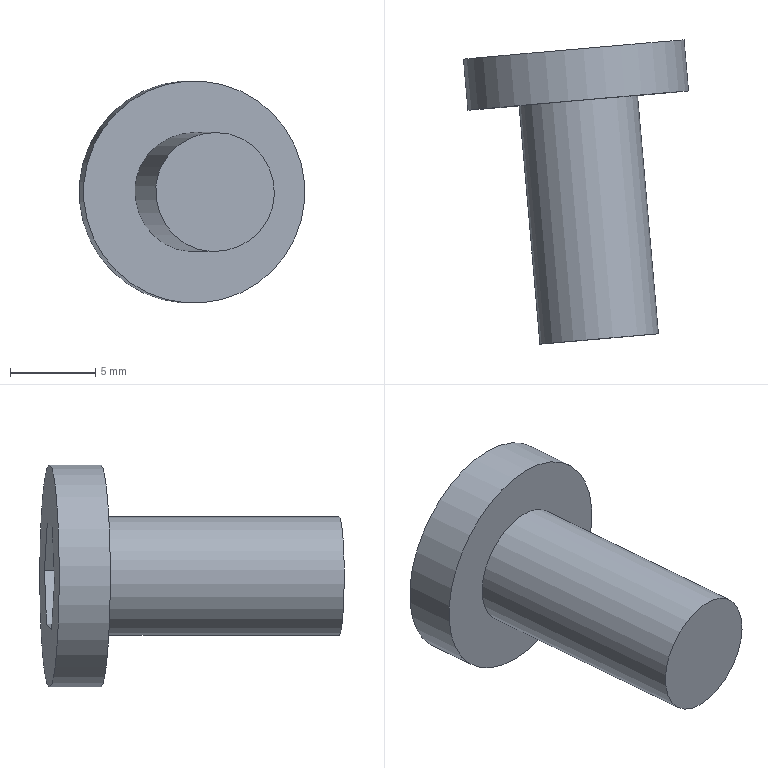Part | NX | features solid 2 | 1 solid | 12 faces | box 13.212 x 17.806 x 13 mm | volume 871.309 mm3 | plane 10 | cylinder 1 | spline 1 | commonest cylinder face diameters 13 x1
STEP:
#1=CARTESIAN_POINT('',(-410.195,38.395,81.103));
#2=VERTEX_POINT('',#1);
#3=CARTESIAN_POINT('',(-416.064,37.882,83.85));
#4=DIRECTION('',(0.08716,-0.9962,0.));
#5=DIRECTION('',(0.9029,0.07899,-0.4226));
#6=AXIS2_PLACEMENT_3D('',#3,#4,#5);
#7=CIRCLE('',#6,6.5);
#8=EDGE_CURVE('',#2,#2,#7,.T.);
#9=ORIENTED_EDGE('',*,*,#8,.F.);
#10=EDGE_LOOP('',(#9));
#11=FACE_BOUND('',#10,.T.);
#12=CARTESIAN_POINT('',(-414.104,38.053,81.041));
#13=VERTEX_POINT('',#12);
#14=CARTESIAN_POINT('',(-412.66,38.18,84.149));
#15=VERTEX_POINT('',#14);
#16=CARTESIAN_POINT('',(-414.104,38.053,81.041));
#17=DIRECTION('',(0.421,0.03683,0.9063));
#18=VECTOR('',#17,1000.);
#19=LINE('',#16,#18);
#20=EDGE_CURVE('',#13,#15,#19,.T.);
#21=ORIENTED_EDGE('',*,*,#20,.T.);
#22=CARTESIAN_POINT('',(-414.62,38.008,86.959));
#23=VERTEX_POINT('',#22);
#24=CARTESIAN_POINT('',(-412.66,38.18,84.149));
#25=DIRECTION('',(-0.5714,-0.04999,0.8192));
#26=VECTOR('',#25,1000.);
#27=LINE('',#24,#26);
#28=EDGE_CURVE('',#15,#23,#27,.T.);
#29=ORIENTED_EDGE('',*,*,#28,.T.);
#30=CARTESIAN_POINT('',(-418.024,37.71,86.66));
#31=VERTEX_POINT('',#30);
#32=CARTESIAN_POINT('',(-414.62,38.008,86.959));
#33=DIRECTION('',(-0.9924,-0.08682,-0.08716));
#34=VECTOR('',#33,1000.);
#35=LINE('',#32,#34);
#36=EDGE_CURVE('',#23,#31,#35,.T.);
#37=ORIENTED_EDGE('',*,*,#36,.T.);
#38=CARTESIAN_POINT('',(-419.468,37.584,83.551));
#39=VERTEX_POINT('',#38);
#40=CARTESIAN_POINT('',(-418.024,37.71,86.66));
#41=DIRECTION('',(-0.421,-0.03683,-0.9063));
#42=VECTOR('',#41,1000.);
#43=LINE('',#40,#42);
#44=EDGE_CURVE('',#31,#39,#43,.T.);
#45=ORIENTED_EDGE('',*,*,#44,.T.);
#46=CARTESIAN_POINT('',(-417.508,37.755,80.742));
#47=VERTEX_POINT('',#46);
#48=CARTESIAN_POINT('',(-419.468,37.584,83.551));
#49=DIRECTION('',(0.5714,0.04999,-0.8192));
#50=VECTOR('',#49,1000.);
#51=LINE('',#48,#50);
#52=EDGE_CURVE('',#39,#47,#51,.T.);
#53=ORIENTED_EDGE('',*,*,#52,.T.);
#54=CARTESIAN_POINT('',(-417.508,37.755,80.742));
#55=DIRECTION('',(0.9924,0.08682,0.08716));
#56=VECTOR('',#55,1000.);
#57=LINE('',#54,#56);
#58=EDGE_CURVE('',#47,#13,#57,.T.);
#59=ORIENTED_EDGE('',*,*,#58,.T.);
#60=EDGE_LOOP('',(#21,#29,#37,#45,#53,#59));
#61=FACE_BOUND('',#60,.T.);
#62=CARTESIAN_POINT('',(-416.064,37.882,83.85));
#63=DIRECTION('',(0.08716,-0.9962,0.));
#64=DIRECTION('',(0.9029,0.07899,-0.4226));
#65=AXIS2_PLACEMENT_3D('',#62,#63,#64);
#66=PLANE('',#65);
#67=ADVANCED_FACE('',(#11,#61),#66,.F.);
#68=CARTESIAN_POINT('',(-409.934,35.407,81.103));
#69=VERTEX_POINT('',#68);
#70=CARTESIAN_POINT('',(-415.802,34.893,83.85));
#71=DIRECTION('',(0.08716,-0.9962,0.));
#72=DIRECTION('',(0.9029,0.07899,-0.4226));
#73=AXIS2_PLACEMENT_3D('',#70,#71,#72);
#74=CIRCLE('',#73,6.5);
#75=EDGE_CURVE('',#69,#69,#74,.T.);
#76=ORIENTED_EDGE('',*,*,#75,.F.);
#77=EDGE_LOOP('',(#76));
#78=FACE_BOUND('',#77,.T.);
#79=ORIENTED_EDGE('',*,*,#8,.T.);
#80=EDGE_LOOP('',(#79));
#81=FACE_BOUND('',#80,.T.);
#82=CARTESIAN_POINT('',(-415.802,34.893,83.85));
#83=DIRECTION('',(-0.08716,0.9962,0.));
#84=DIRECTION('',(-0.9029,-0.07899,0.4226));
#85=AXIS2_PLACEMENT_3D('',#82,#83,#84);
#86=CYLINDRICAL_SURFACE('',#85,6.5);
#87=ADVANCED_FACE('',(#78,#81),#86,.T.);
#88=CARTESIAN_POINT('',(-418.962,34.617,85.33));
#89=VERTEX_POINT('',#88);
#90=CARTESIAN_POINT('',(-419.757,34.547,83.619));
#91=CARTESIAN_POINT('',(-418.168,34.686,87.04));
#92=CARTESIAN_POINT('',(-416.026,34.874,87.815));
#93=CARTESIAN_POINT('',(-412.637,35.17,86.232));
#94=CARTESIAN_POINT('',(-411.852,35.239,84.075));
#95=CARTESIAN_POINT('',(-413.431,35.101,80.672));
#96=CARTESIAN_POINT('',(-415.57,34.914,79.882));
#97=CARTESIAN_POINT('',(-418.974,34.616,81.47));
#98=CARTESIAN_POINT('',(-419.757,34.547,83.619));
#99=CARTESIAN_POINT('',(-418.168,34.686,87.04));
#100=B_SPLINE_CURVE_WITH_KNOTS('',3,(#90,#91,#92,#93,#94,#95,#96,#97,#98,#99),.UNSPECIFIED.,.T.,.F.,(2,2,2,2,2,2,2),(-0.25,0.,0.25,0.5,0.75,1.,1.25),.UNSPECIFIED.);
#101=EDGE_CURVE('',#89,#89,#100,.F.);
#102=ORIENTED_EDGE('',*,*,#101,.F.);
#103=EDGE_LOOP('',(#102));
#104=FACE_BOUND('',#103,.T.);
#105=ORIENTED_EDGE('',*,*,#75,.T.);
#106=EDGE_LOOP('',(#105));
#107=FACE_BOUND('',#106,.T.);
#108=CARTESIAN_POINT('',(-415.802,34.893,83.85));
#109=DIRECTION('',(0.08716,-0.9962,0.));
#110=DIRECTION('',(0.9029,0.07899,-0.4226));
#111=AXIS2_PLACEMENT_3D('',#108,#109,#110);
#112=PLANE('',#111);
#113=ADVANCED_FACE('',(#104,#107),#112,.T.);
#114=ORIENTED_EDGE('',*,*,#20,.F.);
#115=CARTESIAN_POINT('',(-413.93,36.061,81.041));
#116=VERTEX_POINT('',#115);
#117=CARTESIAN_POINT('',(-413.93,36.061,81.041));
#118=DIRECTION('',(-0.08716,0.9962,0.));
#119=VECTOR('',#118,1000.);
#120=LINE('',#117,#119);
#121=EDGE_CURVE('',#116,#13,#120,.T.);
#122=ORIENTED_EDGE('',*,*,#121,.F.);
#123=CARTESIAN_POINT('',(-412.486,36.187,84.149));
#124=VERTEX_POINT('',#123);
#125=CARTESIAN_POINT('',(-413.93,36.061,81.041));
#126=DIRECTION('',(0.421,0.03683,0.9063));
#127=VECTOR('',#126,1000.);
#128=LINE('',#125,#127);
#129=EDGE_CURVE('',#116,#124,#128,.T.);
#130=ORIENTED_EDGE('',*,*,#129,.T.);
#131=CARTESIAN_POINT('',(-412.486,36.187,84.149));
#132=DIRECTION('',(-0.08716,0.9962,0.));
#133=VECTOR('',#132,1000.);
#134=LINE('',#131,#133);
#135=EDGE_CURVE('',#124,#15,#134,.T.);
#136=ORIENTED_EDGE('',*,*,#135,.T.);
#137=EDGE_LOOP('',(#114,#122,#130,#136));
#138=FACE_BOUND('',#137,.T.);
#139=CARTESIAN_POINT('',(-413.93,36.061,81.041));
#140=DIRECTION('',(-0.9029,-0.07899,0.4226));
#141=DIRECTION('',(0.08716,-0.9962,0.));
#142=AXIS2_PLACEMENT_3D('',#139,#140,#141);
#143=PLANE('',#142);
#144=ADVANCED_FACE('',(#138),#143,.T.);
#145=ORIENTED_EDGE('',*,*,#28,.F.);
#146=ORIENTED_EDGE('',*,*,#135,.F.);
#147=CARTESIAN_POINT('',(-414.445,36.016,86.959));
#148=VERTEX_POINT('',#147);
#149=CARTESIAN_POINT('',(-412.486,36.187,84.149));
#150=DIRECTION('',(-0.5714,-0.04999,0.8192));
#151=VECTOR('',#150,1000.);
#152=LINE('',#149,#151);
#153=EDGE_CURVE('',#124,#148,#152,.T.);
#154=ORIENTED_EDGE('',*,*,#153,.T.);
#155=CARTESIAN_POINT('',(-414.445,36.016,86.959));
#156=DIRECTION('',(-0.08716,0.9962,0.));
#157=VECTOR('',#156,1000.);
#158=LINE('',#155,#157);
#159=EDGE_CURVE('',#148,#23,#158,.T.);
#160=ORIENTED_EDGE('',*,*,#159,.T.);
#161=EDGE_LOOP('',(#145,#146,#154,#160));
#162=FACE_BOUND('',#161,.T.);
#163=CARTESIAN_POINT('',(-412.486,36.187,84.149));
#164=DIRECTION('',(-0.816,-0.07139,-0.5736));
#165=DIRECTION('',(0.5714,0.04999,-0.8192));
#166=AXIS2_PLACEMENT_3D('',#163,#164,#165);
#167=PLANE('',#166);
#168=ADVANCED_FACE('',(#162),#167,.T.);
#169=ORIENTED_EDGE('',*,*,#36,.F.);
#170=ORIENTED_EDGE('',*,*,#159,.F.);
#171=CARTESIAN_POINT('',(-417.849,35.718,86.66));
#172=VERTEX_POINT('',#171);
#173=CARTESIAN_POINT('',(-414.445,36.016,86.959));
#174=DIRECTION('',(-0.9924,-0.08682,-0.08716));
#175=VECTOR('',#174,1000.);
#176=LINE('',#173,#175);
#177=EDGE_CURVE('',#148,#172,#176,.T.);
#178=ORIENTED_EDGE('',*,*,#177,.T.);
#179=CARTESIAN_POINT('',(-417.849,35.718,86.66));
#180=DIRECTION('',(-0.08716,0.9962,0.));
#181=VECTOR('',#180,1000.);
#182=LINE('',#179,#181);
#183=EDGE_CURVE('',#172,#31,#182,.T.);
#184=ORIENTED_EDGE('',*,*,#183,.T.);
#185=EDGE_LOOP('',(#169,#170,#178,#184));
#186=FACE_BOUND('',#185,.T.);
#187=CARTESIAN_POINT('',(-414.445,36.016,86.959));
#188=DIRECTION('',(0.08682,0.007596,-0.9962));
#189=DIRECTION('',(0.9924,0.08682,0.08716));
#190=AXIS2_PLACEMENT_3D('',#187,#188,#189);
#191=PLANE('',#190);
#192=ADVANCED_FACE('',(#186),#191,.T.);
#193=ORIENTED_EDGE('',*,*,#44,.F.);
#194=ORIENTED_EDGE('',*,*,#183,.F.);
#195=CARTESIAN_POINT('',(-419.294,35.592,83.551));
#196=VERTEX_POINT('',#195);
#197=CARTESIAN_POINT('',(-417.849,35.718,86.66));
#198=DIRECTION('',(-0.421,-0.03683,-0.9063));
#199=VECTOR('',#198,1000.);
#200=LINE('',#197,#199);
#201=EDGE_CURVE('',#172,#196,#200,.T.);
#202=ORIENTED_EDGE('',*,*,#201,.T.);
#203=CARTESIAN_POINT('',(-419.294,35.592,83.551));
#204=DIRECTION('',(-0.08716,0.9962,0.));
#205=VECTOR('',#204,1000.);
#206=LINE('',#203,#205);
#207=EDGE_CURVE('',#196,#39,#206,.T.);
#208=ORIENTED_EDGE('',*,*,#207,.T.);
#209=EDGE_LOOP('',(#193,#194,#202,#208));
#210=FACE_BOUND('',#209,.T.);
#211=CARTESIAN_POINT('',(-417.849,35.718,86.66));
#212=DIRECTION('',(0.9029,0.07899,-0.4226));
#213=DIRECTION('',(-0.08716,0.9962,0.));
#214=AXIS2_PLACEMENT_3D('',#211,#212,#213);
#215=PLANE('',#214);
#216=ADVANCED_FACE('',(#210),#215,.T.);
#217=ORIENTED_EDGE('',*,*,#52,.F.);
#218=ORIENTED_EDGE('',*,*,#207,.F.);
#219=CARTESIAN_POINT('',(-417.334,35.763,80.742));
#220=VERTEX_POINT('',#219);
#221=CARTESIAN_POINT('',(-419.294,35.592,83.551));
#222=DIRECTION('',(0.5714,0.04999,-0.8192));
#223=VECTOR('',#222,1000.);
#224=LINE('',#221,#223);
#225=EDGE_CURVE('',#196,#220,#224,.T.);
#226=ORIENTED_EDGE('',*,*,#225,.T.);
#227=CARTESIAN_POINT('',(-417.334,35.763,80.742));
#228=DIRECTION('',(-0.08716,0.9962,0.));
#229=VECTOR('',#228,1000.);
#230=LINE('',#227,#229);
#231=EDGE_CURVE('',#220,#47,#230,.T.);
#232=ORIENTED_EDGE('',*,*,#231,.T.);
#233=EDGE_LOOP('',(#217,#218,#226,#232));
#234=FACE_BOUND('',#233,.T.);
#235=CARTESIAN_POINT('',(-419.294,35.592,83.551));
#236=DIRECTION('',(0.816,0.07139,0.5736));
#237=DIRECTION('',(-0.5714,-0.04999,0.8192));
#238=AXIS2_PLACEMENT_3D('',#235,#236,#237);
#239=PLANE('',#238);
#240=ADVANCED_FACE('',(#234),#239,.T.);
#241=ORIENTED_EDGE('',*,*,#58,.F.);
#242=ORIENTED_EDGE('',*,*,#231,.F.);
#243=CARTESIAN_POINT('',(-417.334,35.763,80.742));
#244=DIRECTION('',(0.9924,0.08682,0.08716));
#245=VECTOR('',#244,1000.);
#246=LINE('',#243,#245);
#247=EDGE_CURVE('',#220,#116,#246,.T.);
#248=ORIENTED_EDGE('',*,*,#247,.T.);
#249=ORIENTED_EDGE('',*,*,#121,.T.);
#250=EDGE_LOOP('',(#241,#242,#248,#249));
#251=FACE_BOUND('',#250,.T.);
#252=CARTESIAN_POINT('',(-417.334,35.763,80.742));
#253=DIRECTION('',(-0.08682,-0.007596,0.9962));
#254=DIRECTION('',(-0.9924,-0.08682,-0.08716));
#255=AXIS2_PLACEMENT_3D('',#252,#253,#254);
#256=PLANE('',#255);
#257=ADVANCED_FACE('',(#251),#256,.T.);
#258=ORIENTED_EDGE('',*,*,#129,.F.);
#259=ORIENTED_EDGE('',*,*,#247,.F.);
#260=ORIENTED_EDGE('',*,*,#225,.F.);
#261=ORIENTED_EDGE('',*,*,#201,.F.);
#262=ORIENTED_EDGE('',*,*,#177,.F.);
#263=ORIENTED_EDGE('',*,*,#153,.F.);
#264=EDGE_LOOP('',(#258,#259,#260,#261,#262,#263));
#265=FACE_BOUND('',#264,.T.);
#266=CARTESIAN_POINT('',(-411.042,36.314,87.258));
#267=DIRECTION('',(0.08716,-0.9962,0.));
#268=DIRECTION('',(0.9029,0.07899,-0.4226));
#269=AXIS2_PLACEMENT_3D('',#266,#267,#268);
#270=PLANE('',#269);
#271=ADVANCED_FACE('',(#265),#270,.F.);
#272=CARTESIAN_POINT('',(-417.742,20.67,85.33));
#273=VERTEX_POINT('',#272);
#274=CARTESIAN_POINT('',(-418.537,20.601,83.619));
#275=CARTESIAN_POINT('',(-416.948,20.74,87.04));
#276=CARTESIAN_POINT('',(-414.805,20.927,87.815));
#277=CARTESIAN_POINT('',(-411.416,21.223,86.232));
#278=CARTESIAN_POINT('',(-410.632,21.292,84.075));
#279=CARTESIAN_POINT('',(-412.21,21.154,80.672));
#280=CARTESIAN_POINT('',(-414.35,20.967,79.882));
#281=CARTESIAN_POINT('',(-417.754,20.669,81.47));
#282=CARTESIAN_POINT('',(-418.537,20.601,83.619));
#283=CARTESIAN_POINT('',(-416.948,20.74,87.04));
#284=B_SPLINE_CURVE_WITH_KNOTS('',3,(#274,#275,#276,#277,#278,#279,#280,#281,#282,#283),.UNSPECIFIED.,.T.,.F.,(2,2,2,2,2,2,2),(-0.25,0.,0.25,0.5,0.75,1.,1.25),.UNSPECIFIED.);
#285=EDGE_CURVE('',#273,#273,#284,.T.);
#286=ORIENTED_EDGE('',*,*,#285,.T.);
#287=EDGE_LOOP('',(#286));
#288=FACE_BOUND('',#287,.T.);
#289=ORIENTED_EDGE('',*,*,#101,.T.);
#290=EDGE_LOOP('',(#289));
#291=FACE_BOUND('',#290,.T.);
#292=CARTESIAN_POINT('',(-418.171,20.633,82.535));
#293=CARTESIAN_POINT('',(-419.391,34.579,82.535));
#294=CARTESIAN_POINT('',(-418.099,20.639,85.497));
#295=CARTESIAN_POINT('',(-419.32,34.585,85.497));
#296=CARTESIAN_POINT('',(-415.885,20.833,87.452));
#297=CARTESIAN_POINT('',(-417.105,34.779,87.452));
#298=CARTESIAN_POINT('',(-412.945,21.09,87.382));
#299=CARTESIAN_POINT('',(-414.165,35.036,87.382));
#300=CARTESIAN_POINT('',(-411.,21.26,85.162));
#301=CARTESIAN_POINT('',(-412.22,35.207,85.162));
#302=CARTESIAN_POINT('',(-411.064,21.254,82.206));
#303=CARTESIAN_POINT('',(-412.285,35.201,82.206));
#304=CARTESIAN_POINT('',(-413.271,21.061,80.253));
#305=CARTESIAN_POINT('',(-414.491,35.008,80.253));
#306=CARTESIAN_POINT('',(-416.217,20.803,80.318));
#307=CARTESIAN_POINT('',(-417.437,34.75,80.318));
#308=CARTESIAN_POINT('',(-418.171,20.633,82.535));
#309=CARTESIAN_POINT('',(-419.391,34.579,82.535));
#310=CARTESIAN_POINT('',(-418.099,20.639,85.497));
#311=CARTESIAN_POINT('',(-419.32,34.585,85.497));
#312=CARTESIAN_POINT('',(-415.885,20.833,87.452));
#313=CARTESIAN_POINT('',(-417.105,34.779,87.452));
#314=B_SPLINE_SURFACE_WITH_KNOTS('',3,1,((#292,#293),(#294,#295),(#296,#297),(#298,#299),(#300,#301),(#302,#303),(#304,#305),(#306,#307),(#308,#309),(#310,#311),(#312,#313)),.SURF_OF_LINEAR_EXTRUSION.,.T.,.F.,.F.,(1,1,1,1,1,1,1,1,1,1,1,1,1,1,1),(2,2),(-0.375,-0.25,-0.125,0.,0.125,0.25,0.375,0.5,0.625,0.75,0.875,1.,1.125,1.25,1.375),(0.,1.),.UNSPECIFIED.);
#315=ADVANCED_FACE('',(#288,#291),#314,.T.);
#316=ORIENTED_EDGE('',*,*,#285,.F.);
#317=EDGE_LOOP('',(#316));
#318=FACE_BOUND('',#317,.T.);
#319=CARTESIAN_POINT('',(-411.421,21.223,82.373));
#320=DIRECTION('',(0.08716,-0.9962,0.));
#321=DIRECTION('',(-0.4981,-0.04358,-0.866));
#322=AXIS2_PLACEMENT_3D('',#319,#320,#321);
#323=PLANE('',#322);
#324=ADVANCED_FACE('',(#318),#323,.T.);
#325=CLOSED_SHELL('',(#67,#87,#113,#144,#168,#192,#216,#240,#257,#271,#315,#324));
#326=MANIFOLD_SOLID_BREP('',#325);
#327=(LENGTH_UNIT()NAMED_UNIT(*)SI_UNIT(.MILLI.,.METRE.));
#328=UNCERTAINTY_MEASURE_WITH_UNIT(LENGTH_MEASURE(0.0508),#327,'','');
#329=(NAMED_UNIT(*)PLANE_ANGLE_UNIT()SI_UNIT($,.RADIAN.));
#330=(NAMED_UNIT(*)SI_UNIT($,.STERADIAN.)SOLID_ANGLE_UNIT());
#331=(GEOMETRIC_REPRESENTATION_CONTEXT(3)GLOBAL_UNCERTAINTY_ASSIGNED_CONTEXT((#328))GLOBAL_UNIT_ASSIGNED_CONTEXT((#327,#329,#330))REPRESENTATION_CONTEXT('',''));
#332=ADVANCED_BREP_SHAPE_REPRESENTATION('',(#326),#331);